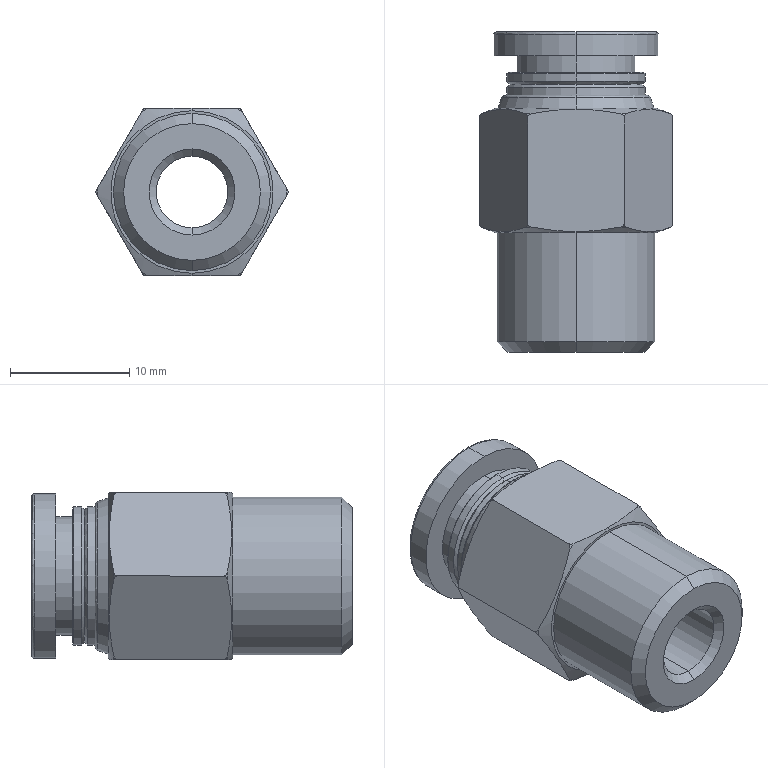Part | STEP file | 11-pc802-V2.0-V2.011 | 1 solid | 62 faces | box 16.166 x 26.8 x 14 mm | volume 2679 mm3 | spline 18 | cone 16 | cylinder 14 | plane 14 | commonest cylinder face diameters 11.6 x4 6 x2 8 x2 9.9 x2 13.157 x2 13.8 x2